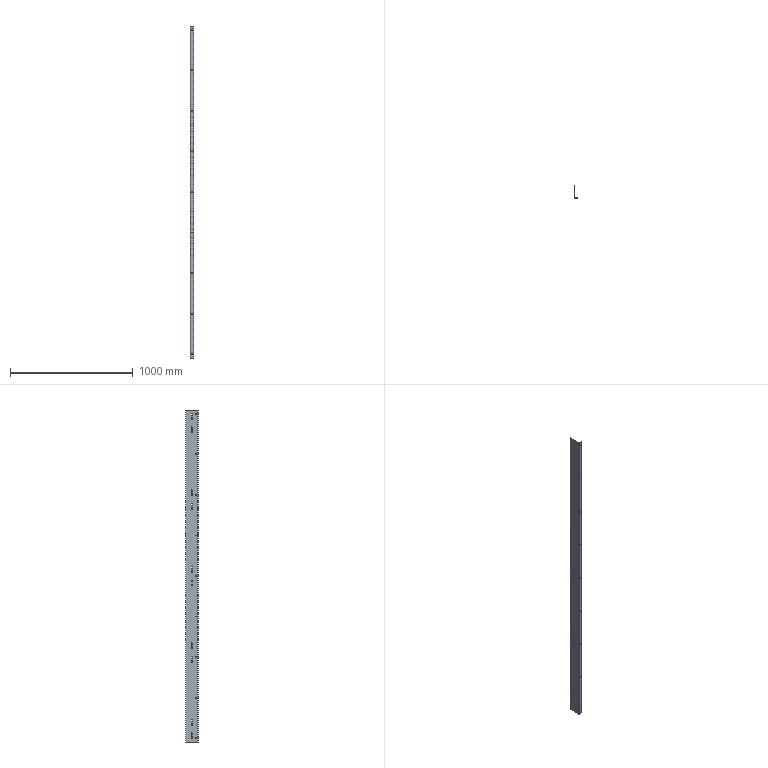Part | STEP file | Angle 85x35x4-2800 GOST 19772-93 | 1 solid | 102 faces | box 32 x 105 x 2700 mm | volume 1063844 mm3 | cylinder 58 | plane 44 | commonest cylinder face diameters 8.2 x38 6.5 x18 4 x1 10 x1